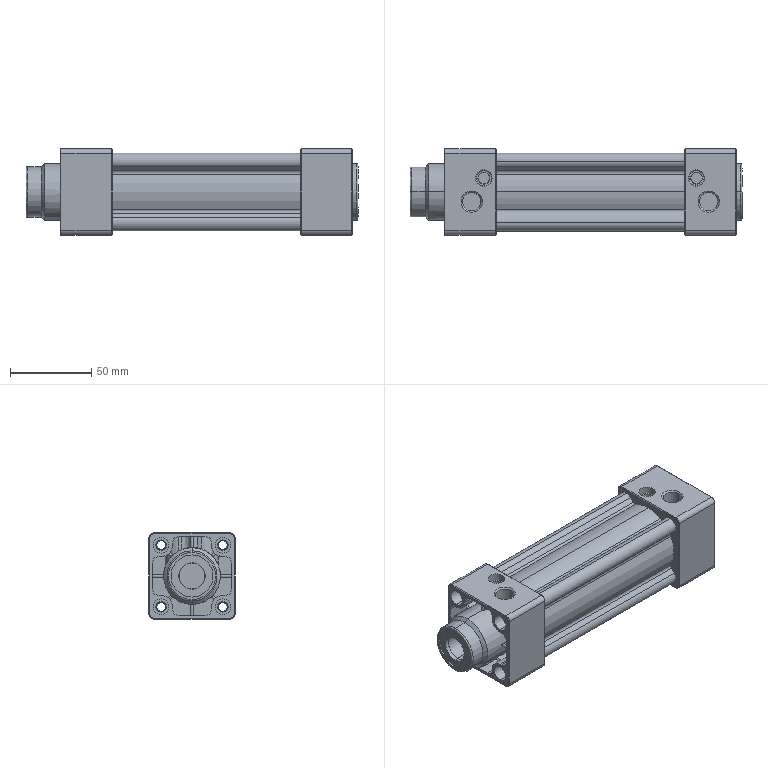Part | STEP file | SI-40X75-S-B1N-2-1 | 1 solid | 349 faces | box 204.5 x 53 x 53 mm | volume 210149 mm3 | cylinder 161 | plane 138 | cone 46 | spline 4 | commonest cylinder face diameters 8 x19 2 x18 6.5 x16 9.7 x16 4 x13 5.3 x8